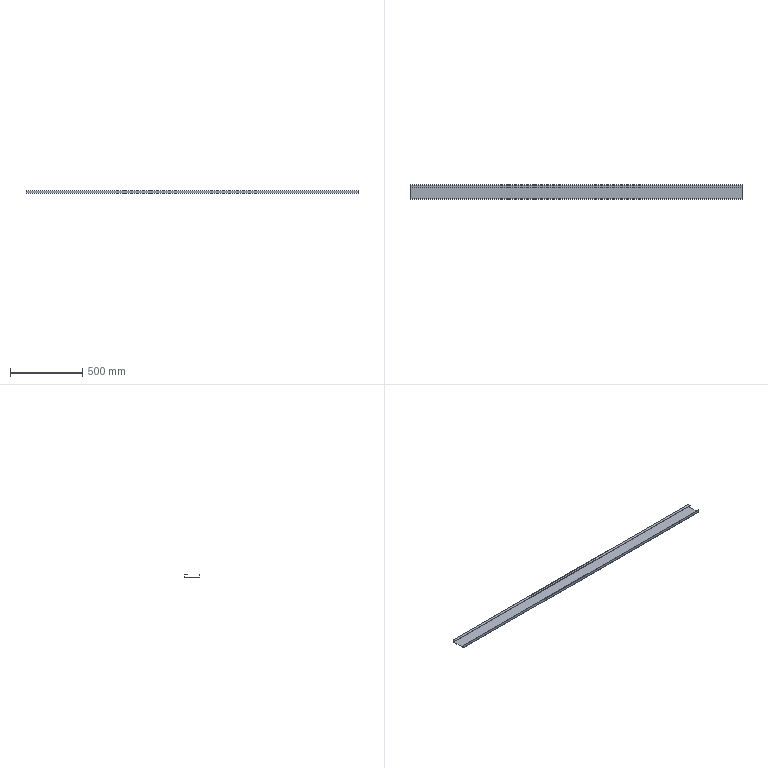Part | STEP file | 粉仓踢脚Plate 6 | 1 solid | 18 faces | box 2290 x 100 x 20 mm | volume 526402 mm3 | plane 12 | cylinder 6 | commonest cylinder face diameters 2 x3 5 x3
STEP:
#1=CARTESIAN_POINT('',(0.,0.,0.));
#2=DIRECTION('',(0.,0.,1.));
#3=DIRECTION('',(1.,0.,0.));
#4=AXIS2_PLACEMENT_3D('',#1,#2,#3);
#5=CARTESIAN_POINT('',(-1145.,1.5,2.5));
#6=VERTEX_POINT('',#5);
#7=CARTESIAN_POINT('',(-1145.,1.5,20.));
#8=VERTEX_POINT('',#7);
#9=CARTESIAN_POINT('',(-1145.,1.5,2.5));
#10=DIRECTION('',(0.,0.,1.));
#11=VECTOR('',#10,1.);
#12=LINE('',#9,#11);
#13=CARTESIAN_POINT('',(1145.,1.5,2.5));
#14=DIRECTION('',(0.,-1.,0.));
#15=DIRECTION('',(0.,0.,-1.));
#16=AXIS2_PLACEMENT_3D('',#13,#14,#15);
#17=PLANE('',#16);
#18=CARTESIAN_POINT('',(0.,-2290.));
#19=DIRECTION('',(-1.,0.));
#20=VECTOR('',#19,1.);
#21=LINE('',#18,#20);
#22=(GEOMETRIC_REPRESENTATION_CONTEXT(2)PARAMETRIC_REPRESENTATION_CONTEXT()REPRESENTATION_CONTEXT('',''));
#23=DEFINITIONAL_REPRESENTATION('',(#21),#22);
#24=PCURVE('',#17,#23);
#25=CARTESIAN_POINT('',(-1145.,2.5,2.5));
#26=DIRECTION('',(-1.,0.,0.));
#27=DIRECTION('',(0.,0.,1.));
#28=AXIS2_PLACEMENT_3D('',#25,#26,#27);
#29=PLANE('',#28);
#30=CARTESIAN_POINT('',(0.,-1.));
#31=DIRECTION('',(1.,0.));
#32=VECTOR('',#31,1.);
#33=LINE('',#30,#32);
#34=(GEOMETRIC_REPRESENTATION_CONTEXT(2)PARAMETRIC_REPRESENTATION_CONTEXT()REPRESENTATION_CONTEXT('',''));
#35=DEFINITIONAL_REPRESENTATION('',(#33),#34);
#36=PCURVE('',#29,#35);
#37=SURFACE_CURVE('',#12,(#24,#36),.PCURVE_S1.);
#38=EDGE_CURVE('',#6,#8,#37,.T.);
#39=ORIENTED_EDGE('',*,*,#38,.T.);
#40=CARTESIAN_POINT('',(1145.,1.5,20.));
#41=VERTEX_POINT('',#40);
#42=CARTESIAN_POINT('',(1145.,1.5,20.));
#43=DIRECTION('',(-1.,0.,0.));
#44=VECTOR('',#43,1.);
#45=LINE('',#42,#44);
#46=CARTESIAN_POINT('',(-17.5,0.));
#47=DIRECTION('',(0.,-1.));
#48=VECTOR('',#47,1.);
#49=LINE('',#46,#48);
#50=(GEOMETRIC_REPRESENTATION_CONTEXT(2)PARAMETRIC_REPRESENTATION_CONTEXT()REPRESENTATION_CONTEXT('',''));
#51=DEFINITIONAL_REPRESENTATION('',(#49),#50);
#52=PCURVE('',#17,#51);
#53=CARTESIAN_POINT('',(1145.,0.,20.));
#54=DIRECTION('',(0.,0.,1.));
#55=DIRECTION('',(1.,0.,0.));
#56=AXIS2_PLACEMENT_3D('',#53,#54,#55);
#57=PLANE('',#56);
#58=CARTESIAN_POINT('',(0.,1.5));
#59=DIRECTION('',(-1.,0.));
#60=VECTOR('',#59,1.);
#61=LINE('',#58,#60);
#62=(GEOMETRIC_REPRESENTATION_CONTEXT(2)PARAMETRIC_REPRESENTATION_CONTEXT()REPRESENTATION_CONTEXT('',''));
#63=DEFINITIONAL_REPRESENTATION('',(#61),#62);
#64=PCURVE('',#57,#63);
#65=SURFACE_CURVE('',#45,(#52,#64),.PCURVE_S1.);
#66=EDGE_CURVE('',#41,#8,#65,.T.);
#67=ORIENTED_EDGE('',*,*,#66,.F.);
#68=CARTESIAN_POINT('',(1145.,1.5,2.5));
#69=VERTEX_POINT('',#68);
#70=CARTESIAN_POINT('',(1145.,1.5,2.5));
#71=DIRECTION('',(0.,0.,1.));
#72=VECTOR('',#71,1.);
#73=LINE('',#70,#72);
#74=CARTESIAN_POINT('',(0.,0.));
#75=DIRECTION('',(-1.,0.));
#76=VECTOR('',#75,1.);
#77=LINE('',#74,#76);
#78=(GEOMETRIC_REPRESENTATION_CONTEXT(2)PARAMETRIC_REPRESENTATION_CONTEXT()REPRESENTATION_CONTEXT('',''));
#79=DEFINITIONAL_REPRESENTATION('',(#77),#78);
#80=PCURVE('',#17,#79);
#81=CARTESIAN_POINT('',(1145.,2.5,2.5));
#82=DIRECTION('',(-1.,0.,0.));
#83=DIRECTION('',(0.,0.,1.));
#84=AXIS2_PLACEMENT_3D('',#81,#82,#83);
#85=PLANE('',#84);
#86=CARTESIAN_POINT('',(0.,-1.));
#87=DIRECTION('',(1.,0.));
#88=VECTOR('',#87,1.);
#89=LINE('',#86,#88);
#90=(GEOMETRIC_REPRESENTATION_CONTEXT(2)PARAMETRIC_REPRESENTATION_CONTEXT()REPRESENTATION_CONTEXT('',''));
#91=DEFINITIONAL_REPRESENTATION('',(#89),#90);
#92=PCURVE('',#85,#91);
#93=SURFACE_CURVE('',#73,(#80,#92),.PCURVE_S1.);
#94=EDGE_CURVE('',#69,#41,#93,.T.);
#95=ORIENTED_EDGE('',*,*,#94,.F.);
#96=CARTESIAN_POINT('',(1145.,1.5,2.5));
#97=DIRECTION('',(-1.,0.,0.));
#98=VECTOR('',#97,1.);
#99=LINE('',#96,#98);
#100=CARTESIAN_POINT('',(0.,0.));
#101=DIRECTION('',(0.,-1.));
#102=VECTOR('',#101,1.);
#103=LINE('',#100,#102);
#104=(GEOMETRIC_REPRESENTATION_CONTEXT(2)PARAMETRIC_REPRESENTATION_CONTEXT()REPRESENTATION_CONTEXT('',''));
#105=DEFINITIONAL_REPRESENTATION('',(#103),#104);
#106=PCURVE('',#17,#105);
#107=CARTESIAN_POINT('',(1145.,2.5,2.5));
#108=DIRECTION('',(-1.,0.,0.));
#109=DIRECTION('',(0.,0.,1.));
#110=AXIS2_PLACEMENT_3D('',#107,#108,#109);
#111=CYLINDRICAL_SURFACE('',#110,1.);
#112=CARTESIAN_POINT('',(4.712,0.));
#113=DIRECTION('',(0.,1.));
#114=VECTOR('',#113,1.);
#115=LINE('',#112,#114);
#116=(GEOMETRIC_REPRESENTATION_CONTEXT(2)PARAMETRIC_REPRESENTATION_CONTEXT()REPRESENTATION_CONTEXT('',''));
#117=DEFINITIONAL_REPRESENTATION('',(#115),#116);
#118=PCURVE('',#111,#117);
#119=SURFACE_CURVE('',#99,(#106,#118),.PCURVE_S1.);
#120=EDGE_CURVE('',#69,#6,#119,.T.);
#121=ORIENTED_EDGE('',*,*,#120,.T.);
#122=EDGE_LOOP('',(#39,#67,#95,#121));
#123=FACE_BOUND('',#122,.T.);
#124=ADVANCED_FACE('',(#123),#17,.F.);
#125=CARTESIAN_POINT('',(-1145.,0.,20.));
#126=VERTEX_POINT('',#125);
#127=CARTESIAN_POINT('',(-1145.,0.,20.));
#128=DIRECTION('',(0.,1.,0.));
#129=VECTOR('',#128,1.);
#130=LINE('',#127,#129);
#131=CARTESIAN_POINT('',(-2290.,0.));
#132=DIRECTION('',(0.,1.));
#133=VECTOR('',#132,1.);
#134=LINE('',#131,#133);
#135=(GEOMETRIC_REPRESENTATION_CONTEXT(2)PARAMETRIC_REPRESENTATION_CONTEXT()REPRESENTATION_CONTEXT('',''));
#136=DEFINITIONAL_REPRESENTATION('',(#134),#135);
#137=PCURVE('',#57,#136);
#138=CARTESIAN_POINT('',(17.5,-2.5));
#139=DIRECTION('',(0.,1.));
#140=VECTOR('',#139,1.);
#141=LINE('',#138,#140);
#142=(GEOMETRIC_REPRESENTATION_CONTEXT(2)PARAMETRIC_REPRESENTATION_CONTEXT()REPRESENTATION_CONTEXT('',''));
#143=DEFINITIONAL_REPRESENTATION('',(#141),#142);
#144=PCURVE('',#29,#143);
#145=SURFACE_CURVE('',#130,(#137,#144),.PCURVE_S1.);
#146=EDGE_CURVE('',#126,#8,#145,.T.);
#147=ORIENTED_EDGE('',*,*,#146,.F.);
#148=CARTESIAN_POINT('',(1145.,0.,20.));
#149=VERTEX_POINT('',#148);
#150=CARTESIAN_POINT('',(1145.,0.,20.));
#151=DIRECTION('',(-1.,0.,0.));
#152=VECTOR('',#151,1.);
#153=LINE('',#150,#152);
#154=CARTESIAN_POINT('',(0.,0.));
#155=DIRECTION('',(-1.,0.));
#156=VECTOR('',#155,1.);
#157=LINE('',#154,#156);
#158=(GEOMETRIC_REPRESENTATION_CONTEXT(2)PARAMETRIC_REPRESENTATION_CONTEXT()REPRESENTATION_CONTEXT('',''));
#159=DEFINITIONAL_REPRESENTATION('',(#157),#158);
#160=PCURVE('',#57,#159);
#161=CARTESIAN_POINT('',(1145.,0.,2.5));
#162=DIRECTION('',(0.,-1.,0.));
#163=DIRECTION('',(0.,0.,-1.));
#164=AXIS2_PLACEMENT_3D('',#161,#162,#163);
#165=PLANE('',#164);
#166=CARTESIAN_POINT('',(-17.5,0.));
#167=DIRECTION('',(0.,-1.));
#168=VECTOR('',#167,1.);
#169=LINE('',#166,#168);
#170=(GEOMETRIC_REPRESENTATION_CONTEXT(2)PARAMETRIC_REPRESENTATION_CONTEXT()REPRESENTATION_CONTEXT('',''));
#171=DEFINITIONAL_REPRESENTATION('',(#169),#170);
#172=PCURVE('',#165,#171);
#173=SURFACE_CURVE('',#153,(#160,#172),.PCURVE_S1.);
#174=EDGE_CURVE('',#149,#126,#173,.T.);
#175=ORIENTED_EDGE('',*,*,#174,.F.);
#176=CARTESIAN_POINT('',(1145.,0.,20.));
#177=DIRECTION('',(0.,1.,0.));
#178=VECTOR('',#177,1.);
#179=LINE('',#176,#178);
#180=CARTESIAN_POINT('',(0.,0.));
#181=DIRECTION('',(0.,1.));
#182=VECTOR('',#181,1.);
#183=LINE('',#180,#182);
#184=(GEOMETRIC_REPRESENTATION_CONTEXT(2)PARAMETRIC_REPRESENTATION_CONTEXT()REPRESENTATION_CONTEXT('',''));
#185=DEFINITIONAL_REPRESENTATION('',(#183),#184);
#186=PCURVE('',#57,#185);
#187=CARTESIAN_POINT('',(17.5,-2.5));
#188=DIRECTION('',(0.,1.));
#189=VECTOR('',#188,1.);
#190=LINE('',#187,#189);
#191=(GEOMETRIC_REPRESENTATION_CONTEXT(2)PARAMETRIC_REPRESENTATION_CONTEXT()REPRESENTATION_CONTEXT('',''));
#192=DEFINITIONAL_REPRESENTATION('',(#190),#191);
#193=PCURVE('',#85,#192);
#194=SURFACE_CURVE('',#179,(#186,#193),.PCURVE_S1.);
#195=EDGE_CURVE('',#149,#41,#194,.T.);
#196=ORIENTED_EDGE('',*,*,#195,.T.);
#197=ORIENTED_EDGE('',*,*,#66,.T.);
#198=EDGE_LOOP('',(#147,#175,#196,#197));
#199=FACE_BOUND('',#198,.T.);
#200=ADVANCED_FACE('',(#199),#57,.T.);
#201=CARTESIAN_POINT('',(-1145.,0.,2.5));
#202=VERTEX_POINT('',#201);
#203=CARTESIAN_POINT('',(-1145.,0.,2.5));
#204=DIRECTION('',(0.,0.,1.));
#205=VECTOR('',#204,1.);
#206=LINE('',#203,#205);
#207=CARTESIAN_POINT('',(0.,-2290.));
#208=DIRECTION('',(-1.,0.));
#209=VECTOR('',#208,1.);
#210=LINE('',#207,#209);
#211=(GEOMETRIC_REPRESENTATION_CONTEXT(2)PARAMETRIC_REPRESENTATION_CONTEXT()REPRESENTATION_CONTEXT('',''));
#212=DEFINITIONAL_REPRESENTATION('',(#210),#211);
#213=PCURVE('',#165,#212);
#214=CARTESIAN_POINT('',(0.,-2.5));
#215=DIRECTION('',(1.,0.));
#216=VECTOR('',#215,1.);
#217=LINE('',#214,#216);
#218=(GEOMETRIC_REPRESENTATION_CONTEXT(2)PARAMETRIC_REPRESENTATION_CONTEXT()REPRESENTATION_CONTEXT('',''));
#219=DEFINITIONAL_REPRESENTATION('',(#217),#218);
#220=PCURVE('',#29,#219);
#221=SURFACE_CURVE('',#206,(#213,#220),.PCURVE_S1.);
#222=EDGE_CURVE('',#202,#126,#221,.T.);
#223=ORIENTED_EDGE('',*,*,#222,.F.);
#224=CARTESIAN_POINT('',(1145.,0.,2.5));
#225=VERTEX_POINT('',#224);
#226=CARTESIAN_POINT('',(1145.,0.,2.5));
#227=DIRECTION('',(-1.,0.,0.));
#228=VECTOR('',#227,1.);
#229=LINE('',#226,#228);
#230=CARTESIAN_POINT('',(0.,0.));
#231=DIRECTION('',(0.,-1.));
#232=VECTOR('',#231,1.);
#233=LINE('',#230,#232);
#234=(GEOMETRIC_REPRESENTATION_CONTEXT(2)PARAMETRIC_REPRESENTATION_CONTEXT()REPRESENTATION_CONTEXT('',''));
#235=DEFINITIONAL_REPRESENTATION('',(#233),#234);
#236=PCURVE('',#165,#235);
#237=CARTESIAN_POINT('',(1145.,2.5,2.5));
#238=DIRECTION('',(-1.,0.,0.));
#239=DIRECTION('',(0.,0.,1.));
#240=AXIS2_PLACEMENT_3D('',#237,#238,#239);
#241=CYLINDRICAL_SURFACE('',#240,2.5);
#242=CARTESIAN_POINT('',(4.712,0.));
#243=DIRECTION('',(0.,1.));
#244=VECTOR('',#243,1.);
#245=LINE('',#242,#244);
#246=(GEOMETRIC_REPRESENTATION_CONTEXT(2)PARAMETRIC_REPRESENTATION_CONTEXT()REPRESENTATION_CONTEXT('',''));
#247=DEFINITIONAL_REPRESENTATION('',(#245),#246);
#248=PCURVE('',#241,#247);
#249=SURFACE_CURVE('',#229,(#236,#248),.PCURVE_S1.);
#250=EDGE_CURVE('',#225,#202,#249,.T.);
#251=ORIENTED_EDGE('',*,*,#250,.F.);
#252=CARTESIAN_POINT('',(1145.,0.,2.5));
#253=DIRECTION('',(0.,0.,1.));
#254=VECTOR('',#253,1.);
#255=LINE('',#252,#254);
#256=CARTESIAN_POINT('',(0.,0.));
#257=DIRECTION('',(-1.,0.));
#258=VECTOR('',#257,1.);
#259=LINE('',#256,#258);
#260=(GEOMETRIC_REPRESENTATION_CONTEXT(2)PARAMETRIC_REPRESENTATION_CONTEXT()REPRESENTATION_CONTEXT('',''));
#261=DEFINITIONAL_REPRESENTATION('',(#259),#260);
#262=PCURVE('',#165,#261);
#263=CARTESIAN_POINT('',(0.,-2.5));
#264=DIRECTION('',(1.,0.));
#265=VECTOR('',#264,1.);
#266=LINE('',#263,#265);
#267=(GEOMETRIC_REPRESENTATION_CONTEXT(2)PARAMETRIC_REPRESENTATION_CONTEXT()REPRESENTATION_CONTEXT('',''));
#268=DEFINITIONAL_REPRESENTATION('',(#266),#267);
#269=PCURVE('',#85,#268);
#270=SURFACE_CURVE('',#255,(#262,#269),.PCURVE_S1.);
#271=EDGE_CURVE('',#225,#149,#270,.T.);
#272=ORIENTED_EDGE('',*,*,#271,.T.);
#273=ORIENTED_EDGE('',*,*,#174,.T.);
#274=EDGE_LOOP('',(#223,#251,#272,#273));
#275=FACE_BOUND('',#274,.T.);
#276=ADVANCED_FACE('',(#275),#165,.T.);
#277=CARTESIAN_POINT('',(-1145.,2.5,0.));
#278=VERTEX_POINT('',#277);
#279=CARTESIAN_POINT('',(-1145.,2.5,2.5));
#280=DIRECTION('',(-1.,0.,0.));
#281=DIRECTION('',(0.,0.,1.));
#282=AXIS2_PLACEMENT_3D('',#279,#280,#281);
#283=CIRCLE('',#282,2.5);
#284=CARTESIAN_POINT('',(0.,2290.));
#285=DIRECTION('',(1.,0.));
#286=VECTOR('',#285,1.);
#287=LINE('',#284,#286);
#288=(GEOMETRIC_REPRESENTATION_CONTEXT(2)PARAMETRIC_REPRESENTATION_CONTEXT()REPRESENTATION_CONTEXT('',''));
#289=DEFINITIONAL_REPRESENTATION('',(#287),#288);
#290=PCURVE('',#241,#289);
#291=CARTESIAN_POINT('',(0.,0.));
#292=DIRECTION('',(1.,0.));
#293=AXIS2_PLACEMENT_2D('',#291,#292);
#294=CIRCLE('',#293,2.5);
#295=(GEOMETRIC_REPRESENTATION_CONTEXT(2)PARAMETRIC_REPRESENTATION_CONTEXT()REPRESENTATION_CONTEXT('',''));
#296=DEFINITIONAL_REPRESENTATION('',(#294),#295);
#297=PCURVE('',#29,#296);
#298=SURFACE_CURVE('',#283,(#290,#297),.PCURVE_S1.);
#299=EDGE_CURVE('',#278,#202,#298,.T.);
#300=ORIENTED_EDGE('',*,*,#299,.F.);
#301=CARTESIAN_POINT('',(1145.,2.5,0.));
#302=VERTEX_POINT('',#301);
#303=CARTESIAN_POINT('',(1145.,2.5,0.));
#304=DIRECTION('',(-1.,0.,0.));
#305=VECTOR('',#304,1.);
#306=LINE('',#303,#305);
#307=CARTESIAN_POINT('',(3.142,0.));
#308=DIRECTION('',(0.,1.));
#309=VECTOR('',#308,1.);
#310=LINE('',#307,#309);
#311=(GEOMETRIC_REPRESENTATION_CONTEXT(2)PARAMETRIC_REPRESENTATION_CONTEXT()REPRESENTATION_CONTEXT('',''));
#312=DEFINITIONAL_REPRESENTATION('',(#310),#311);
#313=PCURVE('',#241,#312);
#314=CARTESIAN_POINT('',(1145.,2.5,0.));
#315=DIRECTION('',(0.,0.,-1.));
#316=DIRECTION('',(-1.,0.,0.));
#317=AXIS2_PLACEMENT_3D('',#314,#315,#316);
#318=PLANE('',#317);
#319=CARTESIAN_POINT('',(0.,0.));
#320=DIRECTION('',(1.,0.));
#321=VECTOR('',#320,1.);
#322=LINE('',#319,#321);
#323=(GEOMETRIC_REPRESENTATION_CONTEXT(2)PARAMETRIC_REPRESENTATION_CONTEXT()REPRESENTATION_CONTEXT('',''));
#324=DEFINITIONAL_REPRESENTATION('',(#322),#323);
#325=PCURVE('',#318,#324);
#326=SURFACE_CURVE('',#306,(#313,#325),.PCURVE_S1.);
#327=EDGE_CURVE('',#302,#278,#326,.T.);
#328=ORIENTED_EDGE('',*,*,#327,.F.);
#329=CARTESIAN_POINT('',(1145.,2.5,2.5));
#330=DIRECTION('',(-1.,0.,0.));
#331=DIRECTION('',(0.,0.,1.));
#332=AXIS2_PLACEMENT_3D('',#329,#330,#331);
#333=CIRCLE('',#332,2.5);
#334=CARTESIAN_POINT('',(0.,0.));
#335=DIRECTION('',(1.,0.));
#336=VECTOR('',#335,1.);
#337=LINE('',#334,#336);
#338=(GEOMETRIC_REPRESENTATION_CONTEXT(2)PARAMETRIC_REPRESENTATION_CONTEXT()REPRESENTATION_CONTEXT('',''));
#339=DEFINITIONAL_REPRESENTATION('',(#337),#338);
#340=PCURVE('',#241,#339);
#341=CARTESIAN_POINT('',(0.,0.));
#342=DIRECTION('',(1.,0.));
#343=AXIS2_PLACEMENT_2D('',#341,#342);
#344=CIRCLE('',#343,2.5);
#345=(GEOMETRIC_REPRESENTATION_CONTEXT(2)PARAMETRIC_REPRESENTATION_CONTEXT()REPRESENTATION_CONTEXT('',''));
#346=DEFINITIONAL_REPRESENTATION('',(#344),#345);
#347=PCURVE('',#85,#346);
#348=SURFACE_CURVE('',#333,(#340,#347),.PCURVE_S1.);
#349=EDGE_CURVE('',#302,#225,#348,.T.);
#350=ORIENTED_EDGE('',*,*,#349,.T.);
#351=ORIENTED_EDGE('',*,*,#250,.T.);
#352=EDGE_LOOP('',(#300,#328,#350,#351));
#353=FACE_BOUND('',#352,.T.);
#354=ADVANCED_FACE('',(#353),#241,.T.);
#355=CARTESIAN_POINT('',(-1145.,97.5,0.));
#356=VERTEX_POINT('',#355);
#357=CARTESIAN_POINT('',(-1145.,2.5,0.));
#358=DIRECTION('',(0.,-1.,0.));
#359=VECTOR('',#358,1.);
#360=LINE('',#357,#359);
#361=CARTESIAN_POINT('',(2290.,0.));
#362=DIRECTION('',(0.,-1.));
#363=VECTOR('',#362,1.);
#364=LINE('',#361,#363);
#365=(GEOMETRIC_REPRESENTATION_CONTEXT(2)PARAMETRIC_REPRESENTATION_CONTEXT()REPRESENTATION_CONTEXT('',''));
#366=DEFINITIONAL_REPRESENTATION('',(#364),#365);
#367=PCURVE('',#318,#366);
#368=CARTESIAN_POINT('',(-2.5,0.));
#369=DIRECTION('',(0.,-1.));
#370=VECTOR('',#369,1.);
#371=LINE('',#368,#370);
#372=(GEOMETRIC_REPRESENTATION_CONTEXT(2)PARAMETRIC_REPRESENTATION_CONTEXT()REPRESENTATION_CONTEXT('',''));
#373=DEFINITIONAL_REPRESENTATION('',(#371),#372);
#374=PCURVE('',#29,#373);
#375=SURFACE_CURVE('',#360,(#367,#374),.PCURVE_S1.);
#376=EDGE_CURVE('',#356,#278,#375,.T.);
#377=ORIENTED_EDGE('',*,*,#376,.F.);
#378=CARTESIAN_POINT('',(1145.,97.5,0.));
#379=VERTEX_POINT('',#378);
#380=CARTESIAN_POINT('',(1145.,97.5,0.));
#381=DIRECTION('',(-1.,0.,0.));
#382=VECTOR('',#381,1.);
#383=LINE('',#380,#382);
#384=CARTESIAN_POINT('',(0.,95.));
#385=DIRECTION('',(1.,0.));
#386=VECTOR('',#385,1.);
#387=LINE('',#384,#386);
#388=(GEOMETRIC_REPRESENTATION_CONTEXT(2)PARAMETRIC_REPRESENTATION_CONTEXT()REPRESENTATION_CONTEXT('',''));
#389=DEFINITIONAL_REPRESENTATION('',(#387),#388);
#390=PCURVE('',#318,#389);
#391=CARTESIAN_POINT('',(1145.,97.5,2.5));
#392=DIRECTION('',(-1.,0.,0.));
#393=DIRECTION('',(0.,0.,1.));
#394=AXIS2_PLACEMENT_3D('',#391,#392,#393);
#395=CYLINDRICAL_SURFACE('',#394,2.5);
#396=CARTESIAN_POINT('',(3.142,0.));
#397=DIRECTION('',(0.,1.));
#398=VECTOR('',#397,1.);
#399=LINE('',#396,#398);
#400=(GEOMETRIC_REPRESENTATION_CONTEXT(2)PARAMETRIC_REPRESENTATION_CONTEXT()REPRESENTATION_CONTEXT('',''));
#401=DEFINITIONAL_REPRESENTATION('',(#399),#400);
#402=PCURVE('',#395,#401);
#403=SURFACE_CURVE('',#383,(#390,#402),.PCURVE_S1.);
#404=EDGE_CURVE('',#379,#356,#403,.T.);
#405=ORIENTED_EDGE('',*,*,#404,.F.);
#406=CARTESIAN_POINT('',(1145.,2.5,0.));
#407=DIRECTION('',(0.,-1.,0.));
#408=VECTOR('',#407,1.);
#409=LINE('',#406,#408);
#410=CARTESIAN_POINT('',(0.,0.));
#411=DIRECTION('',(0.,-1.));
#412=VECTOR('',#411,1.);
#413=LINE('',#410,#412);
#414=(GEOMETRIC_REPRESENTATION_CONTEXT(2)PARAMETRIC_REPRESENTATION_CONTEXT()REPRESENTATION_CONTEXT('',''));
#415=DEFINITIONAL_REPRESENTATION('',(#413),#414);
#416=PCURVE('',#318,#415);
#417=CARTESIAN_POINT('',(-2.5,0.));
#418=DIRECTION('',(0.,-1.));
#419=VECTOR('',#418,1.);
#420=LINE('',#417,#419);
#421=(GEOMETRIC_REPRESENTATION_CONTEXT(2)PARAMETRIC_REPRESENTATION_CONTEXT()REPRESENTATION_CONTEXT('',''));
#422=DEFINITIONAL_REPRESENTATION('',(#420),#421);
#423=PCURVE('',#85,#422);
#424=SURFACE_CURVE('',#409,(#416,#423),.PCURVE_S1.);
#425=EDGE_CURVE('',#379,#302,#424,.T.);
#426=ORIENTED_EDGE('',*,*,#425,.T.);
#427=ORIENTED_EDGE('',*,*,#327,.T.);
#428=EDGE_LOOP('',(#377,#405,#426,#427));
#429=FACE_BOUND('',#428,.T.);
#430=ADVANCED_FACE('',(#429),#318,.T.);
#431=CARTESIAN_POINT('',(-1145.,100.,2.5));
#432=VERTEX_POINT('',#431);
#433=CARTESIAN_POINT('',(-1145.,97.5,2.5));
#434=DIRECTION('',(-1.,0.,0.));
#435=DIRECTION('',(0.,0.,-1.));
#436=AXIS2_PLACEMENT_3D('',#433,#434,#435);
#437=CIRCLE('',#436,2.5);
#438=CARTESIAN_POINT('',(-3.142,2290.));
#439=DIRECTION('',(1.,0.));
#440=VECTOR('',#439,1.);
#441=LINE('',#438,#440);
#442=(GEOMETRIC_REPRESENTATION_CONTEXT(2)PARAMETRIC_REPRESENTATION_CONTEXT()REPRESENTATION_CONTEXT('',''));
#443=DEFINITIONAL_REPRESENTATION('',(#441),#442);
#444=PCURVE('',#395,#443);
#445=CARTESIAN_POINT('',(0.,95.));
#446=DIRECTION('',(-1.,0.));
#447=AXIS2_PLACEMENT_2D('',#445,#446);
#448=CIRCLE('',#447,2.5);
#449=(GEOMETRIC_REPRESENTATION_CONTEXT(2)PARAMETRIC_REPRESENTATION_CONTEXT()REPRESENTATION_CONTEXT('',''));
#450=DEFINITIONAL_REPRESENTATION('',(#448),#449);
#451=PCURVE('',#29,#450);
#452=SURFACE_CURVE('',#437,(#444,#451),.PCURVE_S1.);
#453=EDGE_CURVE('',#432,#356,#452,.T.);
#454=ORIENTED_EDGE('',*,*,#453,.F.);
#455=CARTESIAN_POINT('',(1145.,100.,2.5));
#456=VERTEX_POINT('',#455);
#457=CARTESIAN_POINT('',(1145.,100.,2.5));
#458=DIRECTION('',(-1.,0.,0.));
#459=VECTOR('',#458,1.);
#460=LINE('',#457,#459);
#461=CARTESIAN_POINT('',(1.571,0.));
#462=DIRECTION('',(0.,1.));
#463=VECTOR('',#462,1.);
#464=LINE('',#461,#463);
#465=(GEOMETRIC_REPRESENTATION_CONTEXT(2)PARAMETRIC_REPRESENTATION_CONTEXT()REPRESENTATION_CONTEXT('',''));
#466=DEFINITIONAL_REPRESENTATION('',(#464),#465);
#467=PCURVE('',#395,#466);
#468=CARTESIAN_POINT('',(1145.,100.,2.5));
#469=DIRECTION('',(0.,1.,0.));
#470=DIRECTION('',(0.,0.,1.));
#471=AXIS2_PLACEMENT_3D('',#468,#469,#470);
#472=PLANE('',#471);
#473=CARTESIAN_POINT('',(0.,0.));
#474=DIRECTION('',(0.,-1.));
#475=VECTOR('',#474,1.);
#476=LINE('',#473,#475);
#477=(GEOMETRIC_REPRESENTATION_CONTEXT(2)PARAMETRIC_REPRESENTATION_CONTEXT()REPRESENTATION_CONTEXT('',''));
#478=DEFINITIONAL_REPRESENTATION('',(#476),#477);
#479=PCURVE('',#472,#478);
#480=SURFACE_CURVE('',#460,(#467,#479),.PCURVE_S1.);
#481=EDGE_CURVE('',#456,#432,#480,.T.);
#482=ORIENTED_EDGE('',*,*,#481,.F.);
#483=CARTESIAN_POINT('',(1145.,97.5,2.5));
#484=DIRECTION('',(-1.,0.,0.));
#485=DIRECTION('',(0.,0.,-1.));
#486=AXIS2_PLACEMENT_3D('',#483,#484,#485);
#487=CIRCLE('',#486,2.5);
#488=CARTESIAN_POINT('',(-3.142,0.));
#489=DIRECTION('',(1.,0.));
#490=VECTOR('',#489,1.);
#491=LINE('',#488,#490);
#492=(GEOMETRIC_REPRESENTATION_CONTEXT(2)PARAMETRIC_REPRESENTATION_CONTEXT()REPRESENTATION_CONTEXT('',''));
#493=DEFINITIONAL_REPRESENTATION('',(#491),#492);
#494=PCURVE('',#395,#493);
#495=CARTESIAN_POINT('',(0.,95.));
#496=DIRECTION('',(-1.,0.));
#497=AXIS2_PLACEMENT_2D('',#495,#496);
#498=CIRCLE('',#497,2.5);
#499=(GEOMETRIC_REPRESENTATION_CONTEXT(2)PARAMETRIC_REPRESENTATION_CONTEXT()REPRESENTATION_CONTEXT('',''));
#500=DEFINITIONAL_REPRESENTATION('',(#498),#499);
#501=PCURVE('',#85,#500);
#502=SURFACE_CURVE('',#487,(#494,#501),.PCURVE_S1.);
#503=EDGE_CURVE('',#456,#379,#502,.T.);
#504=ORIENTED_EDGE('',*,*,#503,.T.);
#505=ORIENTED_EDGE('',*,*,#404,.T.);
#506=EDGE_LOOP('',(#454,#482,#504,#505));
#507=FACE_BOUND('',#506,.T.);
#508=ADVANCED_FACE('',(#507),#395,.T.);
#509=CARTESIAN_POINT('',(-1145.,100.,17.5));
#510=VERTEX_POINT('',#509);
#511=CARTESIAN_POINT('',(-1145.,100.,2.5));
#512=DIRECTION('',(0.,0.,-1.));
#513=VECTOR('',#512,1.);
#514=LINE('',#511,#513);
#515=CARTESIAN_POINT('',(0.,-2290.));
#516=DIRECTION('',(-1.,0.));
#517=VECTOR('',#516,1.);
#518=LINE('',#515,#517);
#519=(GEOMETRIC_REPRESENTATION_CONTEXT(2)PARAMETRIC_REPRESENTATION_CONTEXT()REPRESENTATION_CONTEXT('',''));
#520=DEFINITIONAL_REPRESENTATION('',(#518),#519);
#521=PCURVE('',#472,#520);
#522=CARTESIAN_POINT('',(0.,97.5));
#523=DIRECTION('',(-1.,0.));
#524=VECTOR('',#523,1.);
#525=LINE('',#522,#524);
#526=(GEOMETRIC_REPRESENTATION_CONTEXT(2)PARAMETRIC_REPRESENTATION_CONTEXT()REPRESENTATION_CONTEXT('',''));
#527=DEFINITIONAL_REPRESENTATION('',(#525),#526);
#528=PCURVE('',#29,#527);
#529=SURFACE_CURVE('',#514,(#521,#528),.PCURVE_S1.);
#530=EDGE_CURVE('',#510,#432,#529,.T.);
#531=ORIENTED_EDGE('',*,*,#530,.F.);
#532=CARTESIAN_POINT('',(1145.,100.,17.5));
#533=VERTEX_POINT('',#532);
#534=CARTESIAN_POINT('',(1145.,100.,17.5));
#535=DIRECTION('',(-1.,0.,0.));
#536=VECTOR('',#535,1.);
#537=LINE('',#534,#536);
#538=CARTESIAN_POINT('',(15.,0.));
#539=DIRECTION('',(0.,-1.));
#540=VECTOR('',#539,1.);
#541=LINE('',#538,#540);
#542=(GEOMETRIC_REPRESENTATION_CONTEXT(2)PARAMETRIC_REPRESENTATION_CONTEXT()REPRESENTATION_CONTEXT('',''));
#543=DEFINITIONAL_REPRESENTATION('',(#541),#542);
#544=PCURVE('',#472,#543);
#545=CARTESIAN_POINT('',(1145.,97.5,17.5));
#546=DIRECTION('',(-1.,0.,0.));
#547=DIRECTION('',(0.,0.,1.));
#548=AXIS2_PLACEMENT_3D('',#545,#546,#547);
#549=CYLINDRICAL_SURFACE('',#548,2.5);
#550=CARTESIAN_POINT('',(1.571,0.));
#551=DIRECTION('',(0.,1.));
#552=VECTOR('',#551,1.);
#553=LINE('',#550,#552);
#554=(GEOMETRIC_REPRESENTATION_CONTEXT(2)PARAMETRIC_REPRESENTATION_CONTEXT()REPRESENTATION_CONTEXT('',''));
#555=DEFINITIONAL_REPRESENTATION('',(#553),#554);
#556=PCURVE('',#549,#555);
#557=SURFACE_CURVE('',#537,(#544,#556),.PCURVE_S1.);
#558=EDGE_CURVE('',#533,#510,#557,.T.);
#559=ORIENTED_EDGE('',*,*,#558,.F.);
#560=CARTESIAN_POINT('',(1145.,100.,2.5));
#561=DIRECTION('',(0.,0.,-1.));
#562=VECTOR('',#561,1.);
#563=LINE('',#560,#562);
#564=CARTESIAN_POINT('',(0.,0.));
#565=DIRECTION('',(-1.,0.));
#566=VECTOR('',#565,1.);
#567=LINE('',#564,#566);
#568=(GEOMETRIC_REPRESENTATION_CONTEXT(2)PARAMETRIC_REPRESENTATION_CONTEXT()REPRESENTATION_CONTEXT('',''));
#569=DEFINITIONAL_REPRESENTATION('',(#567),#568);
#570=PCURVE('',#472,#569);
#571=CARTESIAN_POINT('',(0.,97.5));
#572=DIRECTION('',(-1.,0.));
#573=VECTOR('',#572,1.);
#574=LINE('',#571,#573);
#575=(GEOMETRIC_REPRESENTATION_CONTEXT(2)PARAMETRIC_REPRESENTATION_CONTEXT()REPRESENTATION_CONTEXT('',''));
#576=DEFINITIONAL_REPRESENTATION('',(#574),#575);
#577=PCURVE('',#85,#576);
#578=SURFACE_CURVE('',#563,(#570,#577),.PCURVE_S1.);
#579=EDGE_CURVE('',#533,#456,#578,.T.);
#580=ORIENTED_EDGE('',*,*,#579,.T.);
#581=ORIENTED_EDGE('',*,*,#481,.T.);
#582=EDGE_LOOP('',(#531,#559,#580,#581));
#583=FACE_BOUND('',#582,.T.);
#584=ADVANCED_FACE('',(#583),#472,.T.);
#585=CARTESIAN_POINT('',(-1145.,97.5,20.));
#586=VERTEX_POINT('',#585);
#587=CARTESIAN_POINT('',(-1145.,97.5,17.5));
#588=DIRECTION('',(-1.,0.,0.));
#589=DIRECTION('',(0.,0.,-1.));
#590=AXIS2_PLACEMENT_3D('',#587,#588,#589);
#591=CIRCLE('',#590,2.5);
#592=CARTESIAN_POINT('',(-3.142,2290.));
#593=DIRECTION('',(1.,0.));
#594=VECTOR('',#593,1.);
#595=LINE('',#592,#594);
#596=(GEOMETRIC_REPRESENTATION_CONTEXT(2)PARAMETRIC_REPRESENTATION_CONTEXT()REPRESENTATION_CONTEXT('',''));
#597=DEFINITIONAL_REPRESENTATION('',(#595),#596);
#598=PCURVE('',#549,#597);
#599=CARTESIAN_POINT('',(15.,95.));
#600=DIRECTION('',(-1.,0.));
#601=AXIS2_PLACEMENT_2D('',#599,#600);
#602=CIRCLE('',#601,2.5);
#603=(GEOMETRIC_REPRESENTATION_CONTEXT(2)PARAMETRIC_REPRESENTATION_CONTEXT()REPRESENTATION_CONTEXT('',''));
#604=DEFINITIONAL_REPRESENTATION('',(#602),#603);
#605=PCURVE('',#29,#604);
#606=SURFACE_CURVE('',#591,(#598,#605),.PCURVE_S1.);
#607=EDGE_CURVE('',#586,#510,#606,.T.);
#608=ORIENTED_EDGE('',*,*,#607,.F.);
#609=CARTESIAN_POINT('',(1145.,97.5,20.));
#610=VERTEX_POINT('',#609);
#611=CARTESIAN_POINT('',(1145.,97.5,20.));
#612=DIRECTION('',(-1.,0.,0.));
#613=VECTOR('',#612,1.);
#614=LINE('',#611,#613);
#615=CARTESIAN_POINT('',(0.,0.));
#616=DIRECTION('',(0.,1.));
#617=VECTOR('',#616,1.);
#618=LINE('',#615,#617);
#619=(GEOMETRIC_REPRESENTATION_CONTEXT(2)PARAMETRIC_REPRESENTATION_CONTEXT()REPRESENTATION_CONTEXT('',''));
#620=DEFINITIONAL_REPRESENTATION('',(#618),#619);
#621=PCURVE('',#549,#620);
#622=CARTESIAN_POINT('',(1145.,97.5,20.));
#623=DIRECTION('',(0.,0.,1.));
#624=DIRECTION('',(1.,0.,0.));
#625=AXIS2_PLACEMENT_3D('',#622,#623,#624);
#626=PLANE('',#625);
#627=CARTESIAN_POINT('',(0.,0.));
#628=DIRECTION('',(-1.,0.));
#629=VECTOR('',#628,1.);
#630=LINE('',#627,#629);
#631=(GEOMETRIC_REPRESENTATION_CONTEXT(2)PARAMETRIC_REPRESENTATION_CONTEXT()REPRESENTATION_CONTEXT('',''));
#632=DEFINITIONAL_REPRESENTATION('',(#630),#631);
#633=PCURVE('',#626,#632);
#634=SURFACE_CURVE('',#614,(#621,#633),.PCURVE_S1.);
#635=EDGE_CURVE('',#610,#586,#634,.T.);
#636=ORIENTED_EDGE('',*,*,#635,.F.);
#637=CARTESIAN_POINT('',(1145.,97.5,17.5));
#638=DIRECTION('',(-1.,0.,0.));
#639=DIRECTION('',(0.,0.,-1.));
#640=AXIS2_PLACEMENT_3D('',#637,#638,#639);
#641=CIRCLE('',#640,2.5);
#642=CARTESIAN_POINT('',(-3.142,0.));
#643=DIRECTION('',(1.,0.));
#644=VECTOR('',#643,1.);
#645=LINE('',#642,#644);
#646=(GEOMETRIC_REPRESENTATION_CONTEXT(2)PARAMETRIC_REPRESENTATION_CONTEXT()REPRESENTATION_CONTEXT('',''));
#647=DEFINITIONAL_REPRESENTATION('',(#645),#646);
#648=PCURVE('',#549,#647);
#649=CARTESIAN_POINT('',(15.,95.));
#650=DIRECTION('',(-1.,0.));
#651=AXIS2_PLACEMENT_2D('',#649,#650);
#652=CIRCLE('',#651,2.5);
#653=(GEOMETRIC_REPRESENTATION_CONTEXT(2)PARAMETRIC_REPRESENTATION_CONTEXT()REPRESENTATION_CONTEXT('',''));
#654=DEFINITIONAL_REPRESENTATION('',(#652),#653);
#655=PCURVE('',#85,#654);
#656=SURFACE_CURVE('',#641,(#648,#655),.PCURVE_S1.);
#657=EDGE_CURVE('',#610,#533,#656,.T.);
#658=ORIENTED_EDGE('',*,*,#657,.T.);
#659=ORIENTED_EDGE('',*,*,#558,.T.);
#660=EDGE_LOOP('',(#608,#636,#658,#659));
#661=FACE_BOUND('',#660,.T.);
#662=ADVANCED_FACE('',(#661),#549,.T.);
#663=CARTESIAN_POINT('',(-1145.,80.,20.));
#664=VERTEX_POINT('',#663);
#665=CARTESIAN_POINT('',(-1145.,97.5,20.));
#666=DIRECTION('',(0.,1.,0.));
#667=VECTOR('',#666,1.);
#668=LINE('',#665,#667);
#669=CARTESIAN_POINT('',(-2290.,0.));
#670=DIRECTION('',(0.,1.));
#671=VECTOR('',#670,1.);
#672=LINE('',#669,#671);
#673=(GEOMETRIC_REPRESENTATION_CONTEXT(2)PARAMETRIC_REPRESENTATION_CONTEXT()REPRESENTATION_CONTEXT('',''));
#674=DEFINITIONAL_REPRESENTATION('',(#672),#673);
#675=PCURVE('',#626,#674);
#676=CARTESIAN_POINT('',(17.5,95.));
#677=DIRECTION('',(0.,1.));
#678=VECTOR('',#677,1.);
#679=LINE('',#676,#678);
#680=(GEOMETRIC_REPRESENTATION_CONTEXT(2)PARAMETRIC_REPRESENTATION_CONTEXT()REPRESENTATION_CONTEXT('',''));
#681=DEFINITIONAL_REPRESENTATION('',(#679),#680);
#682=PCURVE('',#29,#681);
#683=SURFACE_CURVE('',#668,(#675,#682),.PCURVE_S1.);
#684=EDGE_CURVE('',#664,#586,#683,.T.);
#685=ORIENTED_EDGE('',*,*,#684,.F.);
#686=CARTESIAN_POINT('',(1145.,80.,20.));
#687=VERTEX_POINT('',#686);
#688=CARTESIAN_POINT('',(1145.,80.,20.));
#689=DIRECTION('',(-1.,0.,0.));
#690=VECTOR('',#689,1.);
#691=LINE('',#688,#690);
#692=CARTESIAN_POINT('',(0.,-17.5));
#693=DIRECTION('',(-1.,0.));
#694=VECTOR('',#693,1.);
#695=LINE('',#692,#694);
#696=(GEOMETRIC_REPRESENTATION_CONTEXT(2)PARAMETRIC_REPRESENTATION_CONTEXT()REPRESENTATION_CONTEXT('',''));
#697=DEFINITIONAL_REPRESENTATION('',(#695),#696);
#698=PCURVE('',#626,#697);
#699=CARTESIAN_POINT('',(1145.,80.,18.5));
#700=DIRECTION('',(0.,-1.,0.));
#701=DIRECTION('',(0.,0.,-1.));
#702=AXIS2_PLACEMENT_3D('',#699,#700,#701);
#703=PLANE('',#702);
#704=CARTESIAN_POINT('',(-1.5,0.));
#705=DIRECTION('',(0.,-1.));
#706=VECTOR('',#705,1.);
#707=LINE('',#704,#706);
#708=(GEOMETRIC_REPRESENTATION_CONTEXT(2)PARAMETRIC_REPRESENTATION_CONTEXT()REPRESENTATION_CONTEXT('',''));
#709=DEFINITIONAL_REPRESENTATION('',(#707),#708);
#710=PCURVE('',#703,#709);
#711=SURFACE_CURVE('',#691,(#698,#710),.PCURVE_S1.);
#712=EDGE_CURVE('',#687,#664,#711,.T.);
#713=ORIENTED_EDGE('',*,*,#712,.F.);
#714=CARTESIAN_POINT('',(1145.,97.5,20.));
#715=DIRECTION('',(0.,1.,0.));
#716=VECTOR('',#715,1.);
#717=LINE('',#714,#716);
#718=CARTESIAN_POINT('',(0.,0.));
#719=DIRECTION('',(0.,1.));
#720=VECTOR('',#719,1.);
#721=LINE('',#718,#720);
#722=(GEOMETRIC_REPRESENTATION_CONTEXT(2)PARAMETRIC_REPRESENTATION_CONTEXT()REPRESENTATION_CONTEXT('',''));
#723=DEFINITIONAL_REPRESENTATION('',(#721),#722);
#724=PCURVE('',#626,#723);
#725=CARTESIAN_POINT('',(17.5,95.));
#726=DIRECTION('',(0.,1.));
#727=VECTOR('',#726,1.);
#728=LINE('',#725,#727);
#729=(GEOMETRIC_REPRESENTATION_CONTEXT(2)PARAMETRIC_REPRESENTATION_CONTEXT()REPRESENTATION_CONTEXT('',''));
#730=DEFINITIONAL_REPRESENTATION('',(#728),#729);
#731=PCURVE('',#85,#730);
#732=SURFACE_CURVE('',#717,(#724,#731),.PCURVE_S1.);
#733=EDGE_CURVE('',#687,#610,#732,.T.);
#734=ORIENTED_EDGE('',*,*,#733,.T.);
#735=ORIENTED_EDGE('',*,*,#635,.T.);
#736=EDGE_LOOP('',(#685,#713,#734,#735));
#737=FACE_BOUND('',#736,.T.);
#738=ADVANCED_FACE('',(#737),#626,.T.);
#739=CARTESIAN_POINT('',(-1145.,80.,18.5));
#740=VERTEX_POINT('',#739);
#741=CARTESIAN_POINT('',(-1145.,80.,18.5));
#742=DIRECTION('',(0.,0.,1.));
#743=VECTOR('',#742,1.);
#744=LINE('',#741,#743);
#745=CARTESIAN_POINT('',(0.,-2290.));
#746=DIRECTION('',(-1.,0.));
#747=VECTOR('',#746,1.);
#748=LINE('',#745,#747);
#749=(GEOMETRIC_REPRESENTATION_CONTEXT(2)PARAMETRIC_REPRESENTATION_CONTEXT()REPRESENTATION_CONTEXT('',''));
#750=DEFINITIONAL_REPRESENTATION('',(#748),#749);
#751=PCURVE('',#703,#750);
#752=CARTESIAN_POINT('',(16.,77.5));
#753=DIRECTION('',(1.,0.));
#754=VECTOR('',#753,1.);
#755=LINE('',#752,#754);
#756=(GEOMETRIC_REPRESENTATION_CONTEXT(2)PARAMETRIC_REPRESENTATION_CONTEXT()REPRESENTATION_CONTEXT('',''));
#757=DEFINITIONAL_REPRESENTATION('',(#755),#756);
#758=PCURVE('',#29,#757);
#759=SURFACE_CURVE('',#744,(#751,#758),.PCURVE_S1.);
#760=EDGE_CURVE('',#740,#664,#759,.T.);
#761=ORIENTED_EDGE('',*,*,#760,.F.);
#762=CARTESIAN_POINT('',(1145.,80.,18.5));
#763=VERTEX_POINT('',#762);
#764=CARTESIAN_POINT('',(1145.,80.,18.5));
#765=DIRECTION('',(-1.,0.,0.));
#766=VECTOR('',#765,1.);
#767=LINE('',#764,#766);
#768=CARTESIAN_POINT('',(0.,0.));
#769=DIRECTION('',(0.,-1.));
#770=VECTOR('',#769,1.);
#771=LINE('',#768,#770);
#772=(GEOMETRIC_REPRESENTATION_CONTEXT(2)PARAMETRIC_REPRESENTATION_CONTEXT()REPRESENTATION_CONTEXT('',''));
#773=DEFINITIONAL_REPRESENTATION('',(#771),#772);
#774=PCURVE('',#703,#773);
#775=CARTESIAN_POINT('',(1145.,97.5,18.5));
#776=DIRECTION('',(0.,0.,1.));
#777=DIRECTION('',(1.,0.,0.));
#778=AXIS2_PLACEMENT_3D('',#775,#776,#777);
#779=PLANE('',#778);
#780=CARTESIAN_POINT('',(0.,-17.5));
#781=DIRECTION('',(-1.,0.));
#782=VECTOR('',#781,1.);
#783=LINE('',#780,#782);
#784=(GEOMETRIC_REPRESENTATION_CONTEXT(2)PARAMETRIC_REPRESENTATION_CONTEXT()REPRESENTATION_CONTEXT('',''));
#785=DEFINITIONAL_REPRESENTATION('',(#783),#784);
#786=PCURVE('',#779,#785);
#787=SURFACE_CURVE('',#767,(#774,#786),.PCURVE_S1.);
#788=EDGE_CURVE('',#763,#740,#787,.T.);
#789=ORIENTED_EDGE('',*,*,#788,.F.);
#790=CARTESIAN_POINT('',(1145.,80.,18.5));
#791=DIRECTION('',(0.,0.,1.));
#792=VECTOR('',#791,1.);
#793=LINE('',#790,#792);
#794=CARTESIAN_POINT('',(0.,0.));
#795=DIRECTION('',(-1.,0.));
#796=VECTOR('',#795,1.);
#797=LINE('',#794,#796);
#798=(GEOMETRIC_REPRESENTATION_CONTEXT(2)PARAMETRIC_REPRESENTATION_CONTEXT()REPRESENTATION_CONTEXT('',''));
#799=DEFINITIONAL_REPRESENTATION('',(#797),#798);
#800=PCURVE('',#703,#799);
#801=CARTESIAN_POINT('',(16.,77.5));
#802=DIRECTION('',(1.,0.));
#803=VECTOR('',#802,1.);
#804=LINE('',#801,#803);
#805=(GEOMETRIC_REPRESENTATION_CONTEXT(2)PARAMETRIC_REPRESENTATION_CONTEXT()REPRESENTATION_CONTEXT('',''));
#806=DEFINITIONAL_REPRESENTATION('',(#804),#805);
#807=PCURVE('',#85,#806);
#808=SURFACE_CURVE('',#793,(#800,#807),.PCURVE_S1.);
#809=EDGE_CURVE('',#763,#687,#808,.T.);
#810=ORIENTED_EDGE('',*,*,#809,.T.);
#811=ORIENTED_EDGE('',*,*,#712,.T.);
#812=EDGE_LOOP('',(#761,#789,#810,#811));
#813=FACE_BOUND('',#812,.T.);
#814=ADVANCED_FACE('',(#813),#703,.T.);
#815=CARTESIAN_POINT('',(-1145.,97.5,18.5));
#816=VERTEX_POINT('',#815);
#817=CARTESIAN_POINT('',(-1145.,97.5,18.5));
#818=DIRECTION('',(0.,1.,0.));
#819=VECTOR('',#818,1.);
#820=LINE('',#817,#819);
#821=CARTESIAN_POINT('',(-2290.,0.));
#822=DIRECTION('',(0.,1.));
#823=VECTOR('',#822,1.);
#824=LINE('',#821,#823);
#825=(GEOMETRIC_REPRESENTATION_CONTEXT(2)PARAMETRIC_REPRESENTATION_CONTEXT()REPRESENTATION_CONTEXT('',''));
#826=DEFINITIONAL_REPRESENTATION('',(#824),#825);
#827=PCURVE('',#779,#826);
#828=CARTESIAN_POINT('',(16.,95.));
#829=DIRECTION('',(0.,1.));
#830=VECTOR('',#829,1.);
#831=LINE('',#828,#830);
#832=(GEOMETRIC_REPRESENTATION_CONTEXT(2)PARAMETRIC_REPRESENTATION_CONTEXT()REPRESENTATION_CONTEXT('',''));
#833=DEFINITIONAL_REPRESENTATION('',(#831),#832);
#834=PCURVE('',#29,#833);
#835=SURFACE_CURVE('',#820,(#827,#834),.PCURVE_S1.);
#836=EDGE_CURVE('',#740,#816,#835,.T.);
#837=ORIENTED_EDGE('',*,*,#836,.T.);
#838=CARTESIAN_POINT('',(1145.,97.5,18.5));
#839=VERTEX_POINT('',#838);
#840=CARTESIAN_POINT('',(1145.,97.5,18.5));
#841=DIRECTION('',(-1.,0.,0.));
#842=VECTOR('',#841,1.);
#843=LINE('',#840,#842);
#844=CARTESIAN_POINT('',(0.,0.));
#845=DIRECTION('',(-1.,0.));
#846=VECTOR('',#845,1.);
#847=LINE('',#844,#846);
#848=(GEOMETRIC_REPRESENTATION_CONTEXT(2)PARAMETRIC_REPRESENTATION_CONTEXT()REPRESENTATION_CONTEXT('',''));
#849=DEFINITIONAL_REPRESENTATION('',(#847),#848);
#850=PCURVE('',#779,#849);
#851=CARTESIAN_POINT('',(1145.,97.5,17.5));
#852=DIRECTION('',(-1.,0.,0.));
#853=DIRECTION('',(0.,0.,1.));
#854=AXIS2_PLACEMENT_3D('',#851,#852,#853);
#855=CYLINDRICAL_SURFACE('',#854,1.);
#856=CARTESIAN_POINT('',(0.,0.));
#857=DIRECTION('',(0.,1.));
#858=VECTOR('',#857,1.);
#859=LINE('',#856,#858);
#860=(GEOMETRIC_REPRESENTATION_CONTEXT(2)PARAMETRIC_REPRESENTATION_CONTEXT()REPRESENTATION_CONTEXT('',''));
#861=DEFINITIONAL_REPRESENTATION('',(#859),#860);
#862=PCURVE('',#855,#861);
#863=SURFACE_CURVE('',#843,(#850,#862),.PCURVE_S1.);
#864=EDGE_CURVE('',#839,#816,#863,.T.);
#865=ORIENTED_EDGE('',*,*,#864,.F.);
#866=CARTESIAN_POINT('',(1145.,97.5,18.5));
#867=DIRECTION('',(0.,1.,0.));
#868=VECTOR('',#867,1.);
#869=LINE('',#866,#868);
#870=CARTESIAN_POINT('',(0.,0.));
#871=DIRECTION('',(0.,1.));
#872=VECTOR('',#871,1.);
#873=LINE('',#870,#872);
#874=(GEOMETRIC_REPRESENTATION_CONTEXT(2)PARAMETRIC_REPRESENTATION_CONTEXT()REPRESENTATION_CONTEXT('',''));
#875=DEFINITIONAL_REPRESENTATION('',(#873),#874);
#876=PCURVE('',#779,#875);
#877=CARTESIAN_POINT('',(16.,95.));
#878=DIRECTION('',(0.,1.));
#879=VECTOR('',#878,1.);
#880=LINE('',#877,#879);
#881=(GEOMETRIC_REPRESENTATION_CONTEXT(2)PARAMETRIC_REPRESENTATION_CONTEXT()REPRESENTATION_CONTEXT('',''));
#882=DEFINITIONAL_REPRESENTATION('',(#880),#881);
#883=PCURVE('',#85,#882);
#884=SURFACE_CURVE('',#869,(#876,#883),.PCURVE_S1.);
#885=EDGE_CURVE('',#763,#839,#884,.T.);
#886=ORIENTED_EDGE('',*,*,#885,.F.);
#887=ORIENTED_EDGE('',*,*,#788,.T.);
#888=EDGE_LOOP('',(#837,#865,#886,#887));
#889=FACE_BOUND('',#888,.T.);
#890=ADVANCED_FACE('',(#889),#779,.F.);
#891=ORIENTED_EDGE('',*,*,#864,.F.);
#892=CARTESIAN_POINT('',(1145.,98.5,17.5));
#893=VERTEX_POINT('',#892);
#894=CARTESIAN_POINT('',(1145.,97.5,17.5));
#895=DIRECTION('',(-1.,0.,0.));
#896=DIRECTION('',(0.,0.,-1.));
#897=AXIS2_PLACEMENT_3D('',#894,#895,#896);
#898=CIRCLE('',#897,1.);
#899=CARTESIAN_POINT('',(-3.142,0.));
#900=DIRECTION('',(1.,0.));
#901=VECTOR('',#900,1.);
#902=LINE('',#899,#901);
#903=(GEOMETRIC_REPRESENTATION_CONTEXT(2)PARAMETRIC_REPRESENTATION_CONTEXT()REPRESENTATION_CONTEXT('',''));
#904=DEFINITIONAL_REPRESENTATION('',(#902),#903);
#905=PCURVE('',#855,#904);
#906=CARTESIAN_POINT('',(15.,95.));
#907=DIRECTION('',(-1.,0.));
#908=AXIS2_PLACEMENT_2D('',#906,#907);
#909=CIRCLE('',#908,1.);
#910=(GEOMETRIC_REPRESENTATION_CONTEXT(2)PARAMETRIC_REPRESENTATION_CONTEXT()REPRESENTATION_CONTEXT('',''));
#911=DEFINITIONAL_REPRESENTATION('',(#909),#910);
#912=PCURVE('',#85,#911);
#913=SURFACE_CURVE('',#898,(#905,#912),.PCURVE_S1.);
#914=EDGE_CURVE('',#839,#893,#913,.T.);
#915=ORIENTED_EDGE('',*,*,#914,.T.);
#916=CARTESIAN_POINT('',(-1145.,98.5,17.5));
#917=VERTEX_POINT('',#916);
#918=CARTESIAN_POINT('',(1145.,98.5,17.5));
#919=DIRECTION('',(-1.,0.,0.));
#920=VECTOR('',#919,1.);
#921=LINE('',#918,#920);
#922=CARTESIAN_POINT('',(1.571,0.));
#923=DIRECTION('',(0.,1.));
#924=VECTOR('',#923,1.);
#925=LINE('',#922,#924);
#926=(GEOMETRIC_REPRESENTATION_CONTEXT(2)PARAMETRIC_REPRESENTATION_CONTEXT()REPRESENTATION_CONTEXT('',''));
#927=DEFINITIONAL_REPRESENTATION('',(#925),#926);
#928=PCURVE('',#855,#927);
#929=CARTESIAN_POINT('',(1145.,98.5,2.5));
#930=DIRECTION('',(0.,1.,0.));
#931=DIRECTION('',(0.,0.,1.));
#932=AXIS2_PLACEMENT_3D('',#929,#930,#931);
#933=PLANE('',#932);
#934=CARTESIAN_POINT('',(15.,0.));
#935=DIRECTION('',(0.,-1.));
#936=VECTOR('',#935,1.);
#937=LINE('',#934,#936);
#938=(GEOMETRIC_REPRESENTATION_CONTEXT(2)PARAMETRIC_REPRESENTATION_CONTEXT()REPRESENTATION_CONTEXT('',''));
#939=DEFINITIONAL_REPRESENTATION('',(#937),#938);
#940=PCURVE('',#933,#939);
#941=SURFACE_CURVE('',#921,(#928,#940),.PCURVE_S1.);
#942=EDGE_CURVE('',#893,#917,#941,.T.);
#943=ORIENTED_EDGE('',*,*,#942,.T.);
#944=CARTESIAN_POINT('',(-1145.,97.5,17.5));
#945=DIRECTION('',(-1.,0.,0.));
#946=DIRECTION('',(0.,0.,-1.));
#947=AXIS2_PLACEMENT_3D('',#944,#945,#946);
#948=CIRCLE('',#947,1.);
#949=CARTESIAN_POINT('',(-3.142,2290.));
#950=DIRECTION('',(1.,0.));
#951=VECTOR('',#950,1.);
#952=LINE('',#949,#951);
#953=(GEOMETRIC_REPRESENTATION_CONTEXT(2)PARAMETRIC_REPRESENTATION_CONTEXT()REPRESENTATION_CONTEXT('',''));
#954=DEFINITIONAL_REPRESENTATION('',(#952),#953);
#955=PCURVE('',#855,#954);
#956=CARTESIAN_POINT('',(15.,95.));
#957=DIRECTION('',(-1.,0.));
#958=AXIS2_PLACEMENT_2D('',#956,#957);
#959=CIRCLE('',#958,1.);
#960=(GEOMETRIC_REPRESENTATION_CONTEXT(2)PARAMETRIC_REPRESENTATION_CONTEXT()REPRESENTATION_CONTEXT('',''));
#961=DEFINITIONAL_REPRESENTATION('',(#959),#960);
#962=PCURVE('',#29,#961);
#963=SURFACE_CURVE('',#948,(#955,#962),.PCURVE_S1.);
#964=EDGE_CURVE('',#816,#917,#963,.T.);
#965=ORIENTED_EDGE('',*,*,#964,.F.);
#966=EDGE_LOOP('',(#891,#915,#943,#965));
#967=FACE_BOUND('',#966,.F.);
#968=ADVANCED_FACE('',(#967),#855,.F.);
#969=CARTESIAN_POINT('',(-1145.,98.5,2.5));
#970=VERTEX_POINT('',#969);
#971=CARTESIAN_POINT('',(-1145.,98.5,2.5));
#972=DIRECTION('',(0.,0.,-1.));
#973=VECTOR('',#972,1.);
#974=LINE('',#971,#973);
#975=CARTESIAN_POINT('',(0.,-2290.));
#976=DIRECTION('',(-1.,0.));
#977=VECTOR('',#976,1.);
#978=LINE('',#975,#977);
#979=(GEOMETRIC_REPRESENTATION_CONTEXT(2)PARAMETRIC_REPRESENTATION_CONTEXT()REPRESENTATION_CONTEXT('',''));
#980=DEFINITIONAL_REPRESENTATION('',(#978),#979);
#981=PCURVE('',#933,#980);
#982=CARTESIAN_POINT('',(0.,96.));
#983=DIRECTION('',(-1.,0.));
#984=VECTOR('',#983,1.);
#985=LINE('',#982,#984);
#986=(GEOMETRIC_REPRESENTATION_CONTEXT(2)PARAMETRIC_REPRESENTATION_CONTEXT()REPRESENTATION_CONTEXT('',''));
#987=DEFINITIONAL_REPRESENTATION('',(#985),#986);
#988=PCURVE('',#29,#987);
#989=SURFACE_CURVE('',#974,(#981,#988),.PCURVE_S1.);
#990=EDGE_CURVE('',#917,#970,#989,.T.);
#991=ORIENTED_EDGE('',*,*,#990,.T.);
#992=CARTESIAN_POINT('',(1145.,98.5,2.5));
#993=VERTEX_POINT('',#992);
#994=CARTESIAN_POINT('',(1145.,98.5,2.5));
#995=DIRECTION('',(-1.,0.,0.));
#996=VECTOR('',#995,1.);
#997=LINE('',#994,#996);
#998=CARTESIAN_POINT('',(0.,0.));
#999=DIRECTION('',(0.,-1.));
#1000=VECTOR('',#999,1.);
#1001=LINE('',#998,#1000);
#1002=(GEOMETRIC_REPRESENTATION_CONTEXT(2)PARAMETRIC_REPRESENTATION_CONTEXT()REPRESENTATION_CONTEXT('',''));
#1003=DEFINITIONAL_REPRESENTATION('',(#1001),#1002);
#1004=PCURVE('',#933,#1003);
#1005=CARTESIAN_POINT('',(1145.,97.5,2.5));
#1006=DIRECTION('',(-1.,0.,0.));
#1007=DIRECTION('',(0.,0.,1.));
#1008=AXIS2_PLACEMENT_3D('',#1005,#1006,#1007);
#1009=CYLINDRICAL_SURFACE('',#1008,1.);
#1010=CARTESIAN_POINT('',(1.571,0.));
#1011=DIRECTION('',(0.,1.));
#1012=VECTOR('',#1011,1.);
#1013=LINE('',#1010,#1012);
#1014=(GEOMETRIC_REPRESENTATION_CONTEXT(2)PARAMETRIC_REPRESENTATION_CONTEXT()REPRESENTATION_CONTEXT('',''));
#1015=DEFINITIONAL_REPRESENTATION('',(#1013),#1014);
#1016=PCURVE('',#1009,#1015);
#1017=SURFACE_CURVE('',#997,(#1004,#1016),.PCURVE_S1.);
#1018=EDGE_CURVE('',#993,#970,#1017,.T.);
#1019=ORIENTED_EDGE('',*,*,#1018,.F.);
#1020=CARTESIAN_POINT('',(1145.,98.5,2.5));
#1021=DIRECTION('',(0.,0.,-1.));
#1022=VECTOR('',#1021,1.);
#1023=LINE('',#1020,#1022);
#1024=CARTESIAN_POINT('',(0.,0.));
#1025=DIRECTION('',(-1.,0.));
#1026=VECTOR('',#1025,1.);
#1027=LINE('',#1024,#1026);
#1028=(GEOMETRIC_REPRESENTATION_CONTEXT(2)PARAMETRIC_REPRESENTATION_CONTEXT()REPRESENTATION_CONTEXT('',''));
#1029=DEFINITIONAL_REPRESENTATION('',(#1027),#1028);
#1030=PCURVE('',#933,#1029);
#1031=CARTESIAN_POINT('',(0.,96.));
#1032=DIRECTION('',(-1.,0.));
#1033=VECTOR('',#1032,1.);
#1034=LINE('',#1031,#1033);
#1035=(GEOMETRIC_REPRESENTATION_CONTEXT(2)PARAMETRIC_REPRESENTATION_CONTEXT()REPRESENTATION_CONTEXT('',''));
#1036=DEFINITIONAL_REPRESENTATION('',(#1034),#1035);
#1037=PCURVE('',#85,#1036);
#1038=SURFACE_CURVE('',#1023,(#1030,#1037),.PCURVE_S1.);
#1039=EDGE_CURVE('',#893,#993,#1038,.T.);
#1040=ORIENTED_EDGE('',*,*,#1039,.F.);
#1041=ORIENTED_EDGE('',*,*,#942,.T.);
#1042=EDGE_LOOP('',(#991,#1019,#1040,#1041));
#1043=FACE_BOUND('',#1042,.T.);
#1044=ADVANCED_FACE('',(#1043),#933,.F.);
#1045=ORIENTED_EDGE('',*,*,#1018,.F.);
#1046=CARTESIAN_POINT('',(1145.,97.5,1.5));
#1047=VERTEX_POINT('',#1046);
#1048=CARTESIAN_POINT('',(1145.,97.5,2.5));
#1049=DIRECTION('',(-1.,0.,0.));
#1050=DIRECTION('',(0.,0.,-1.));
#1051=AXIS2_PLACEMENT_3D('',#1048,#1049,#1050);
#1052=CIRCLE('',#1051,1.);
#1053=CARTESIAN_POINT('',(-3.142,0.));
#1054=DIRECTION('',(1.,0.));
#1055=VECTOR('',#1054,1.);
#1056=LINE('',#1053,#1055);
#1057=(GEOMETRIC_REPRESENTATION_CONTEXT(2)PARAMETRIC_REPRESENTATION_CONTEXT()REPRESENTATION_CONTEXT('',''));
#1058=DEFINITIONAL_REPRESENTATION('',(#1056),#1057);
#1059=PCURVE('',#1009,#1058);
#1060=CARTESIAN_POINT('',(0.,95.));
#1061=DIRECTION('',(-1.,0.));
#1062=AXIS2_PLACEMENT_2D('',#1060,#1061);
#1063=CIRCLE('',#1062,1.);
#1064=(GEOMETRIC_REPRESENTATION_CONTEXT(2)PARAMETRIC_REPRESENTATION_CONTEXT()REPRESENTATION_CONTEXT('',''));
#1065=DEFINITIONAL_REPRESENTATION('',(#1063),#1064);
#1066=PCURVE('',#85,#1065);
#1067=SURFACE_CURVE('',#1052,(#1059,#1066),.PCURVE_S1.);
#1068=EDGE_CURVE('',#993,#1047,#1067,.T.);
#1069=ORIENTED_EDGE('',*,*,#1068,.T.);
#1070=CARTESIAN_POINT('',(-1145.,97.5,1.5));
#1071=VERTEX_POINT('',#1070);
#1072=CARTESIAN_POINT('',(1145.,97.5,1.5));
#1073=DIRECTION('',(-1.,0.,0.));
#1074=VECTOR('',#1073,1.);
#1075=LINE('',#1072,#1074);
#1076=CARTESIAN_POINT('',(3.142,0.));
#1077=DIRECTION('',(0.,1.));
#1078=VECTOR('',#1077,1.);
#1079=LINE('',#1076,#1078);
#1080=(GEOMETRIC_REPRESENTATION_CONTEXT(2)PARAMETRIC_REPRESENTATION_CONTEXT()REPRESENTATION_CONTEXT('',''));
#1081=DEFINITIONAL_REPRESENTATION('',(#1079),#1080);
#1082=PCURVE('',#1009,#1081);
#1083=CARTESIAN_POINT('',(1145.,2.5,1.5));
#1084=DIRECTION('',(0.,0.,-1.));
#1085=DIRECTION('',(-1.,0.,0.));
#1086=AXIS2_PLACEMENT_3D('',#1083,#1084,#1085);
#1087=PLANE('',#1086);
#1088=CARTESIAN_POINT('',(0.,95.));
#1089=DIRECTION('',(1.,0.));
#1090=VECTOR('',#1089,1.);
#1091=LINE('',#1088,#1090);
#1092=(GEOMETRIC_REPRESENTATION_CONTEXT(2)PARAMETRIC_REPRESENTATION_CONTEXT()REPRESENTATION_CONTEXT('',''));
#1093=DEFINITIONAL_REPRESENTATION('',(#1091),#1092);
#1094=PCURVE('',#1087,#1093);
#1095=SURFACE_CURVE('',#1075,(#1082,#1094),.PCURVE_S1.);
#1096=EDGE_CURVE('',#1047,#1071,#1095,.T.);
#1097=ORIENTED_EDGE('',*,*,#1096,.T.);
#1098=CARTESIAN_POINT('',(-1145.,97.5,2.5));
#1099=DIRECTION('',(-1.,0.,0.));
#1100=DIRECTION('',(0.,0.,-1.));
#1101=AXIS2_PLACEMENT_3D('',#1098,#1099,#1100);
#1102=CIRCLE('',#1101,1.);
#1103=CARTESIAN_POINT('',(-3.142,2290.));
#1104=DIRECTION('',(1.,0.));
#1105=VECTOR('',#1104,1.);
#1106=LINE('',#1103,#1105);
#1107=(GEOMETRIC_REPRESENTATION_CONTEXT(2)PARAMETRIC_REPRESENTATION_CONTEXT()REPRESENTATION_CONTEXT('',''));
#1108=DEFINITIONAL_REPRESENTATION('',(#1106),#1107);
#1109=PCURVE('',#1009,#1108);
#1110=CARTESIAN_POINT('',(0.,95.));
#1111=DIRECTION('',(-1.,0.));
#1112=AXIS2_PLACEMENT_2D('',#1110,#1111);
#1113=CIRCLE('',#1112,1.);
#1114=(GEOMETRIC_REPRESENTATION_CONTEXT(2)PARAMETRIC_REPRESENTATION_CONTEXT()REPRESENTATION_CONTEXT('',''));
#1115=DEFINITIONAL_REPRESENTATION('',(#1113),#1114);
#1116=PCURVE('',#29,#1115);
#1117=SURFACE_CURVE('',#1102,(#1109,#1116),.PCURVE_S1.);
#1118=EDGE_CURVE('',#970,#1071,#1117,.T.);
#1119=ORIENTED_EDGE('',*,*,#1118,.F.);
#1120=EDGE_LOOP('',(#1045,#1069,#1097,#1119));
#1121=FACE_BOUND('',#1120,.F.);
#1122=ADVANCED_FACE('',(#1121),#1009,.F.);
#1123=CARTESIAN_POINT('',(-1145.,2.5,1.5));
#1124=VERTEX_POINT('',#1123);
#1125=CARTESIAN_POINT('',(-1145.,2.5,1.5));
#1126=DIRECTION('',(0.,-1.,0.));
#1127=VECTOR('',#1126,1.);
#1128=LINE('',#1125,#1127);
#1129=CARTESIAN_POINT('',(2290.,0.));
#1130=DIRECTION('',(0.,-1.));
#1131=VECTOR('',#1130,1.);
#1132=LINE('',#1129,#1131);
#1133=(GEOMETRIC_REPRESENTATION_CONTEXT(2)PARAMETRIC_REPRESENTATION_CONTEXT()REPRESENTATION_CONTEXT('',''));
#1134=DEFINITIONAL_REPRESENTATION('',(#1132),#1133);
#1135=PCURVE('',#1087,#1134);
#1136=CARTESIAN_POINT('',(-1.,0.));
#1137=DIRECTION('',(0.,-1.));
#1138=VECTOR('',#1137,1.);
#1139=LINE('',#1136,#1138);
#1140=(GEOMETRIC_REPRESENTATION_CONTEXT(2)PARAMETRIC_REPRESENTATION_CONTEXT()REPRESENTATION_CONTEXT('',''));
#1141=DEFINITIONAL_REPRESENTATION('',(#1139),#1140);
#1142=PCURVE('',#29,#1141);
#1143=SURFACE_CURVE('',#1128,(#1135,#1142),.PCURVE_S1.);
#1144=EDGE_CURVE('',#1071,#1124,#1143,.T.);
#1145=ORIENTED_EDGE('',*,*,#1144,.T.);
#1146=CARTESIAN_POINT('',(1145.,2.5,1.5));
#1147=VERTEX_POINT('',#1146);
#1148=CARTESIAN_POINT('',(1145.,2.5,1.5));
#1149=DIRECTION('',(-1.,0.,0.));
#1150=VECTOR('',#1149,1.);
#1151=LINE('',#1148,#1150);
#1152=CARTESIAN_POINT('',(0.,0.));
#1153=DIRECTION('',(1.,0.));
#1154=VECTOR('',#1153,1.);
#1155=LINE('',#1152,#1154);
#1156=(GEOMETRIC_REPRESENTATION_CONTEXT(2)PARAMETRIC_REPRESENTATION_CONTEXT()REPRESENTATION_CONTEXT('',''));
#1157=DEFINITIONAL_REPRESENTATION('',(#1155),#1156);
#1158=PCURVE('',#1087,#1157);
#1159=CARTESIAN_POINT('',(3.142,0.));
#1160=DIRECTION('',(0.,1.));
#1161=VECTOR('',#1160,1.);
#1162=LINE('',#1159,#1161);
#1163=(GEOMETRIC_REPRESENTATION_CONTEXT(2)PARAMETRIC_REPRESENTATION_CONTEXT()REPRESENTATION_CONTEXT('',''));
#1164=DEFINITIONAL_REPRESENTATION('',(#1162),#1163);
#1165=PCURVE('',#111,#1164);
#1166=SURFACE_CURVE('',#1151,(#1158,#1165),.PCURVE_S1.);
#1167=EDGE_CURVE('',#1147,#1124,#1166,.T.);
#1168=ORIENTED_EDGE('',*,*,#1167,.F.);
#1169=CARTESIAN_POINT('',(1145.,2.5,1.5));
#1170=DIRECTION('',(0.,-1.,0.));
#1171=VECTOR('',#1170,1.);
#1172=LINE('',#1169,#1171);
#1173=CARTESIAN_POINT('',(0.,0.));
#1174=DIRECTION('',(0.,-1.));
#1175=VECTOR('',#1174,1.);
#1176=LINE('',#1173,#1175);
#1177=(GEOMETRIC_REPRESENTATION_CONTEXT(2)PARAMETRIC_REPRESENTATION_CONTEXT()REPRESENTATION_CONTEXT('',''));
#1178=DEFINITIONAL_REPRESENTATION('',(#1176),#1177);
#1179=PCURVE('',#1087,#1178);
#1180=CARTESIAN_POINT('',(-1.,0.));
#1181=DIRECTION('',(0.,-1.));
#1182=VECTOR('',#1181,1.);
#1183=LINE('',#1180,#1182);
#1184=(GEOMETRIC_REPRESENTATION_CONTEXT(2)PARAMETRIC_REPRESENTATION_CONTEXT()REPRESENTATION_CONTEXT('',''));
#1185=DEFINITIONAL_REPRESENTATION('',(#1183),#1184);
#1186=PCURVE('',#85,#1185);
#1187=SURFACE_CURVE('',#1172,(#1179,#1186),.PCURVE_S1.);
#1188=EDGE_CURVE('',#1047,#1147,#1187,.T.);
#1189=ORIENTED_EDGE('',*,*,#1188,.F.);
#1190=ORIENTED_EDGE('',*,*,#1096,.T.);
#1191=EDGE_LOOP('',(#1145,#1168,#1189,#1190));
#1192=FACE_BOUND('',#1191,.T.);
#1193=ADVANCED_FACE('',(#1192),#1087,.F.);
#1194=ORIENTED_EDGE('',*,*,#1167,.F.);
#1195=CARTESIAN_POINT('',(1145.,2.5,2.5));
#1196=DIRECTION('',(-1.,0.,0.));
#1197=DIRECTION('',(0.,0.,-1.));
#1198=AXIS2_PLACEMENT_3D('',#1195,#1196,#1197);
#1199=CIRCLE('',#1198,1.);
#1200=CARTESIAN_POINT('',(3.142,0.));
#1201=DIRECTION('',(1.,0.));
#1202=VECTOR('',#1201,1.);
#1203=LINE('',#1200,#1202);
#1204=(GEOMETRIC_REPRESENTATION_CONTEXT(2)PARAMETRIC_REPRESENTATION_CONTEXT()REPRESENTATION_CONTEXT('',''));
#1205=DEFINITIONAL_REPRESENTATION('',(#1203),#1204);
#1206=PCURVE('',#111,#1205);
#1207=CARTESIAN_POINT('',(0.,0.));
#1208=DIRECTION('',(-1.,0.));
#1209=AXIS2_PLACEMENT_2D('',#1207,#1208);
#1210=CIRCLE('',#1209,1.);
#1211=(GEOMETRIC_REPRESENTATION_CONTEXT(2)PARAMETRIC_REPRESENTATION_CONTEXT()REPRESENTATION_CONTEXT('',''));
#1212=DEFINITIONAL_REPRESENTATION('',(#1210),#1211);
#1213=PCURVE('',#85,#1212);
#1214=SURFACE_CURVE('',#1199,(#1206,#1213),.PCURVE_S1.);
#1215=EDGE_CURVE('',#1147,#69,#1214,.T.);
#1216=ORIENTED_EDGE('',*,*,#1215,.T.);
#1217=ORIENTED_EDGE('',*,*,#120,.T.);
#1218=CARTESIAN_POINT('',(-1145.,2.5,2.5));
#1219=DIRECTION('',(-1.,0.,0.));
#1220=DIRECTION('',(0.,0.,-1.));
#1221=AXIS2_PLACEMENT_3D('',#1218,#1219,#1220);
#1222=CIRCLE('',#1221,1.);
#1223=CARTESIAN_POINT('',(3.142,2290.));
#1224=DIRECTION('',(1.,0.));
#1225=VECTOR('',#1224,1.);
#1226=LINE('',#1223,#1225);
#1227=(GEOMETRIC_REPRESENTATION_CONTEXT(2)PARAMETRIC_REPRESENTATION_CONTEXT()REPRESENTATION_CONTEXT('',''));
#1228=DEFINITIONAL_REPRESENTATION('',(#1226),#1227);
#1229=PCURVE('',#111,#1228);
#1230=CARTESIAN_POINT('',(0.,0.));
#1231=DIRECTION('',(-1.,0.));
#1232=AXIS2_PLACEMENT_2D('',#1230,#1231);
#1233=CIRCLE('',#1232,1.);
#1234=(GEOMETRIC_REPRESENTATION_CONTEXT(2)PARAMETRIC_REPRESENTATION_CONTEXT()REPRESENTATION_CONTEXT('',''));
#1235=DEFINITIONAL_REPRESENTATION('',(#1233),#1234);
#1236=PCURVE('',#29,#1235);
#1237=SURFACE_CURVE('',#1222,(#1229,#1236),.PCURVE_S1.);
#1238=EDGE_CURVE('',#1124,#6,#1237,.T.);
#1239=ORIENTED_EDGE('',*,*,#1238,.F.);
#1240=EDGE_LOOP('',(#1194,#1216,#1217,#1239));
#1241=FACE_BOUND('',#1240,.F.);
#1242=ADVANCED_FACE('',(#1241),#111,.F.);
#1243=ORIENTED_EDGE('',*,*,#94,.T.);
#1244=ORIENTED_EDGE('',*,*,#195,.F.);
#1245=ORIENTED_EDGE('',*,*,#271,.F.);
#1246=ORIENTED_EDGE('',*,*,#349,.F.);
#1247=ORIENTED_EDGE('',*,*,#425,.F.);
#1248=ORIENTED_EDGE('',*,*,#503,.F.);
#1249=ORIENTED_EDGE('',*,*,#579,.F.);
#1250=ORIENTED_EDGE('',*,*,#657,.F.);
#1251=ORIENTED_EDGE('',*,*,#733,.F.);
#1252=ORIENTED_EDGE('',*,*,#809,.F.);
#1253=ORIENTED_EDGE('',*,*,#885,.T.);
#1254=ORIENTED_EDGE('',*,*,#914,.T.);
#1255=ORIENTED_EDGE('',*,*,#1039,.T.);
#1256=ORIENTED_EDGE('',*,*,#1068,.T.);
#1257=ORIENTED_EDGE('',*,*,#1188,.T.);
#1258=ORIENTED_EDGE('',*,*,#1215,.T.);
#1259=EDGE_LOOP('',(#1243,#1244,#1245,#1246,#1247,#1248,#1249,#1250,#1251,#1252,#1253,#1254,#1255,#1256,#1257,#1258));
#1260=FACE_BOUND('',#1259,.T.);
#1261=ADVANCED_FACE('',(#1260),#85,.F.);
#1262=ORIENTED_EDGE('',*,*,#38,.F.);
#1263=ORIENTED_EDGE('',*,*,#1238,.F.);
#1264=ORIENTED_EDGE('',*,*,#1144,.F.);
#1265=ORIENTED_EDGE('',*,*,#1118,.F.);
#1266=ORIENTED_EDGE('',*,*,#990,.F.);
#1267=ORIENTED_EDGE('',*,*,#964,.F.);
#1268=ORIENTED_EDGE('',*,*,#836,.F.);
#1269=ORIENTED_EDGE('',*,*,#760,.T.);
#1270=ORIENTED_EDGE('',*,*,#684,.T.);
#1271=ORIENTED_EDGE('',*,*,#607,.T.);
#1272=ORIENTED_EDGE('',*,*,#530,.T.);
#1273=ORIENTED_EDGE('',*,*,#453,.T.);
#1274=ORIENTED_EDGE('',*,*,#376,.T.);
#1275=ORIENTED_EDGE('',*,*,#299,.T.);
#1276=ORIENTED_EDGE('',*,*,#222,.T.);
#1277=ORIENTED_EDGE('',*,*,#146,.T.);
#1278=EDGE_LOOP('',(#1262,#1263,#1264,#1265,#1266,#1267,#1268,#1269,#1270,#1271,#1272,#1273,#1274,#1275,#1276,#1277));
#1279=FACE_BOUND('',#1278,.T.);
#1280=ADVANCED_FACE('',(#1279),#29,.T.);
#1281=CLOSED_SHELL('',(#124,#200,#276,#354,#430,#508,#584,#662,#738,#814,#890,#968,#1044,#1122,#1193,#1242,#1261,#1280));
#1282=MANIFOLD_SOLID_BREP('',#1281);
#1283=(LENGTH_UNIT()NAMED_UNIT(*)SI_UNIT(.MILLI.,.METRE.));
#1284=UNCERTAINTY_MEASURE_WITH_UNIT(LENGTH_MEASURE(0.0000001),#1283,'','');
#1285=(NAMED_UNIT(*)PLANE_ANGLE_UNIT()SI_UNIT($,.RADIAN.));
#1286=(NAMED_UNIT(*)SI_UNIT($,.STERADIAN.)SOLID_ANGLE_UNIT());
#1287=(GEOMETRIC_REPRESENTATION_CONTEXT(3)GLOBAL_UNCERTAINTY_ASSIGNED_CONTEXT((#1284))GLOBAL_UNIT_ASSIGNED_CONTEXT((#1283,#1285,#1286))REPRESENTATION_CONTEXT('',''));
#1288=ADVANCED_BREP_SHAPE_REPRESENTATION('',(#4,#1282),#1287);